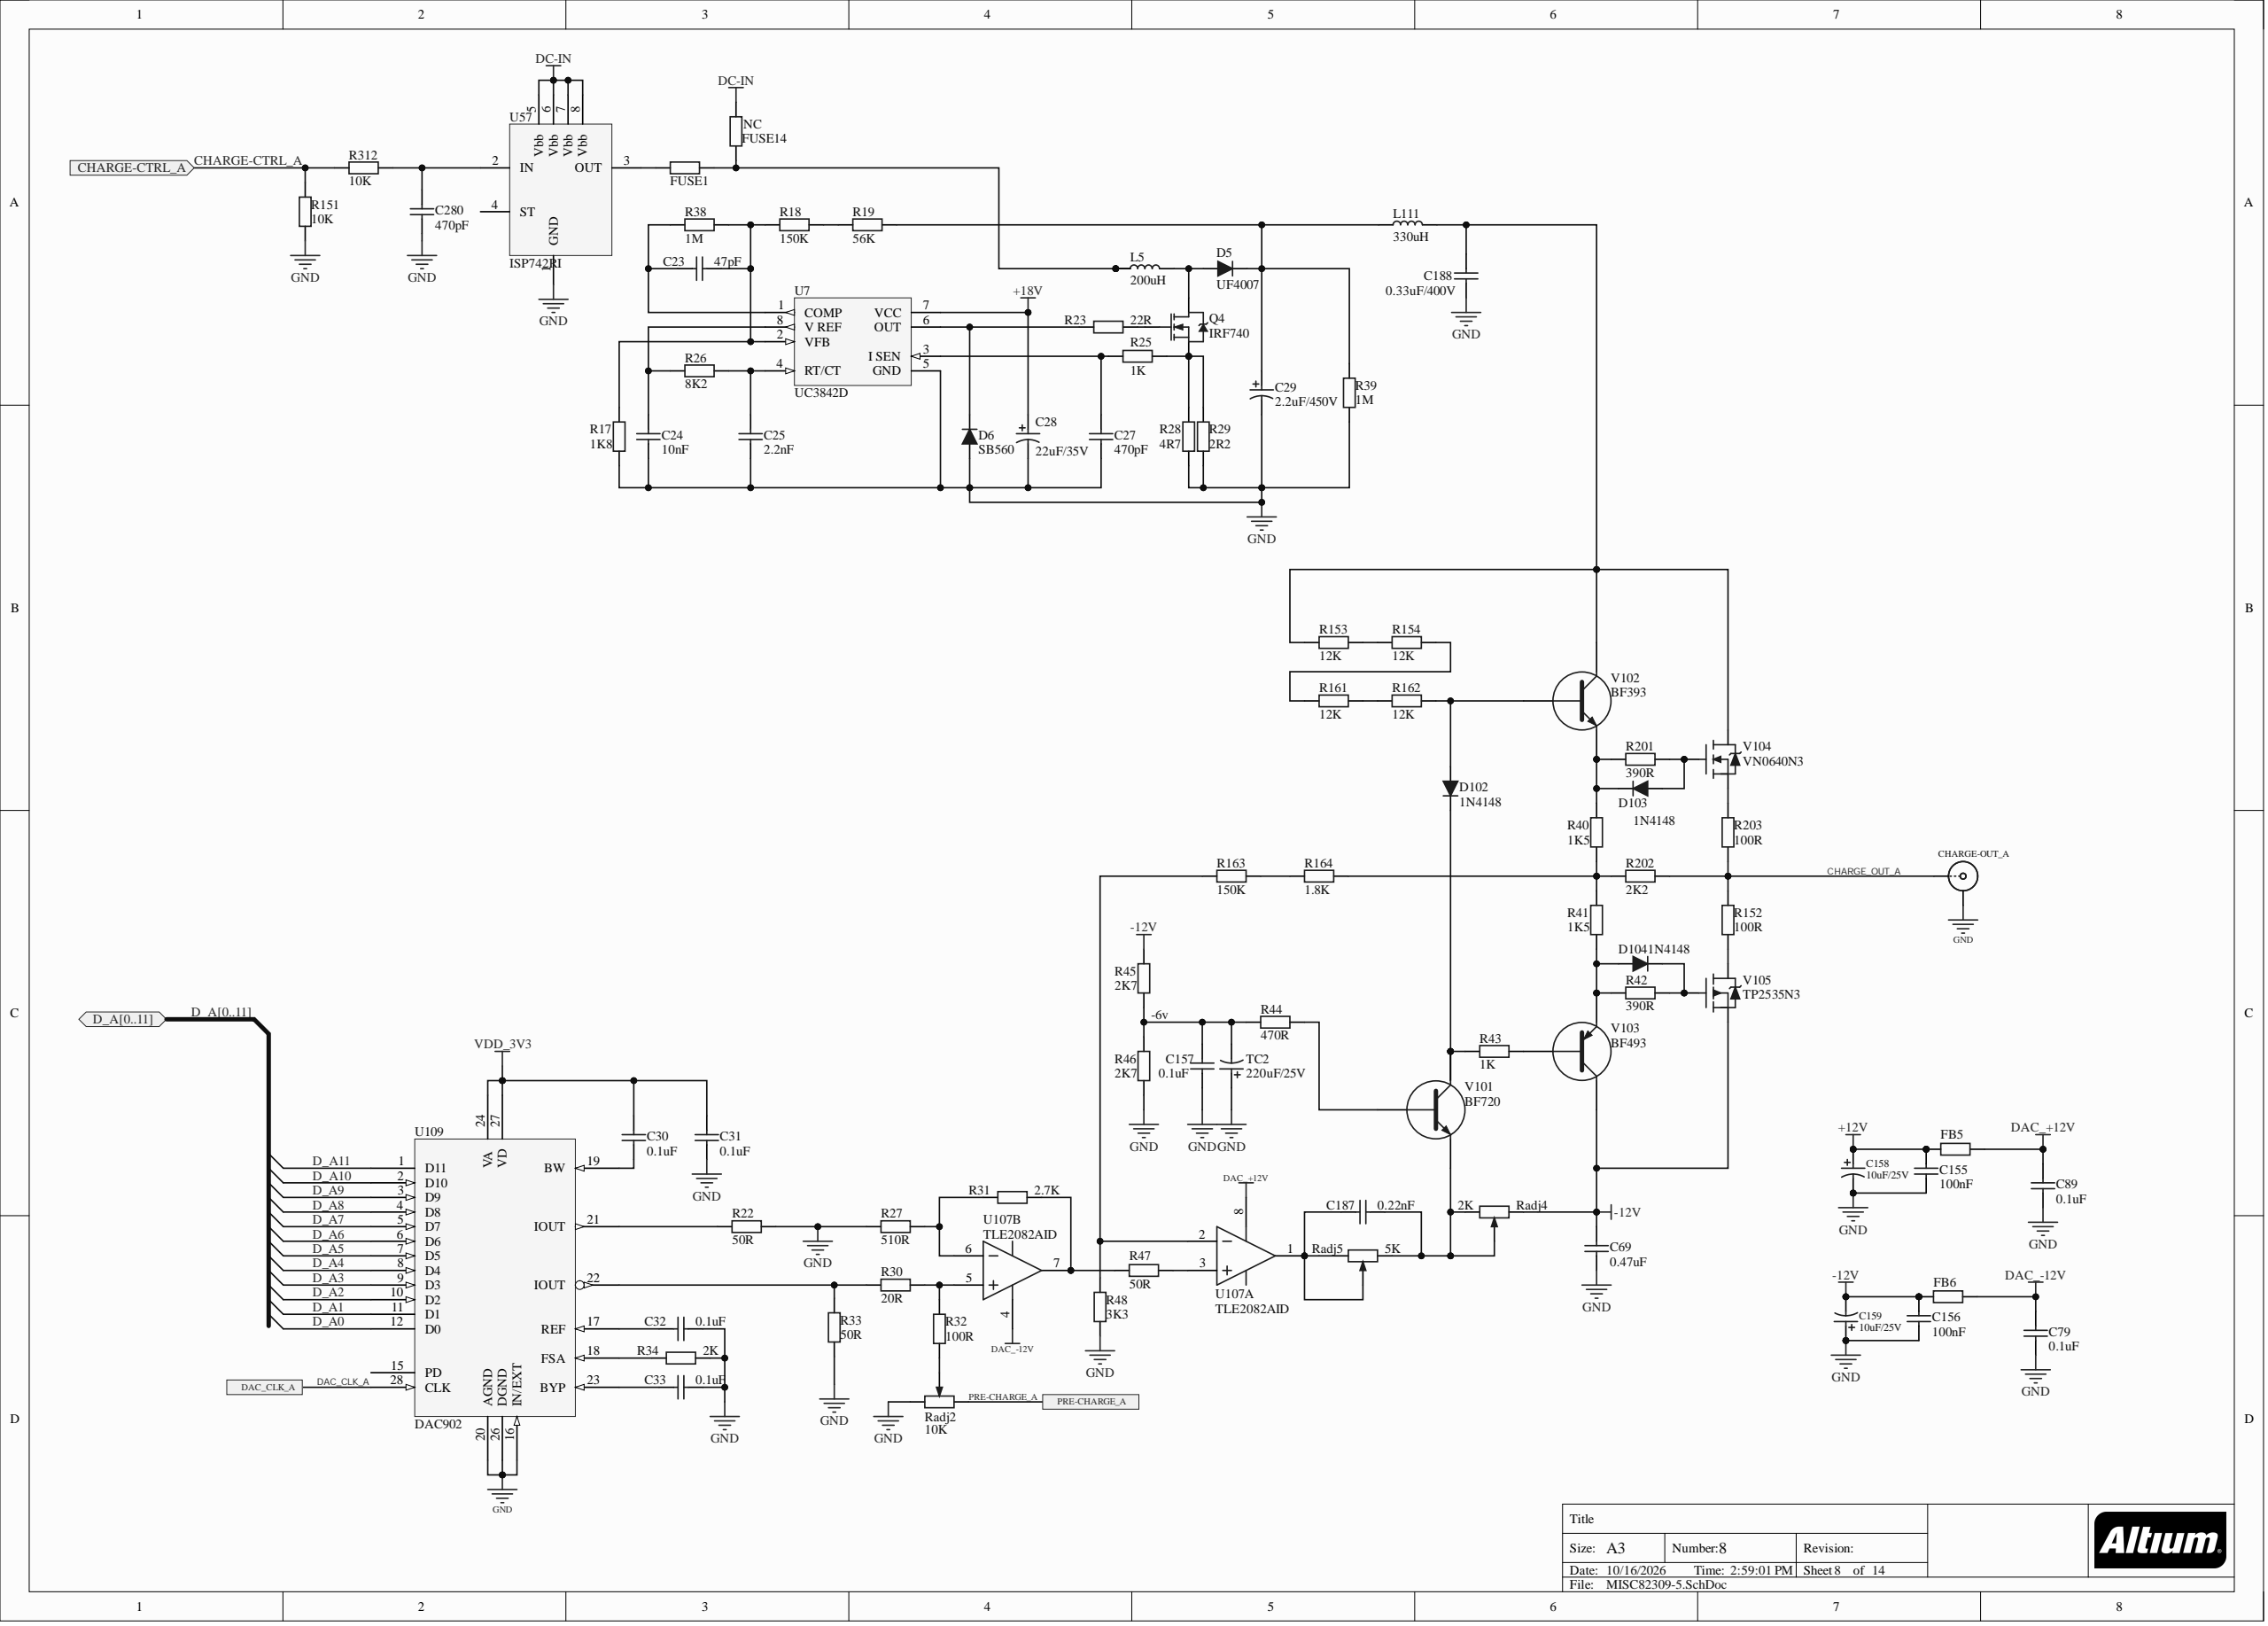Circuit board | Altium Designer | 747 parts | 576 nets | one sheet of the schematic
Parts on this sheet (reference | value | footprint):
C23 | 47pF | C1206
C24 | 10nF | C1206
C25 | 2.2nF | C1206
C27 | 470pF | C1206
C28 | 22uF/35V | E6.3X5.4
C29 | 2.2uF/450V | CAP-EL-10X13_5-5
C30 | 0.1uF | CAP_0805
C31 | 0.1uF | CAP_0805
C32 | 0.1uF | CAP_0805
C33 | 0.1uF | CAP_0805
C69 | 0.47uF | C1206
C79 | 0.1uF | C0805
C89 | 0.1uF | C0805
C155 | 100nF | C0805
C156 | 100nF | C0805
C157 | 0.1uF | CAP_0805
C158 | 10uF/25V | E5X5.4
C159 | 10uF/25V | E5X5.4
C187 | 0.22nF | CAP_0805
C188 | 0.33uF/400V | CBB-400V-10mm
C280 | 470pF | C0603
CHARGE-OUT_A | SMB | SMB_V-RJ45
D102 | 1N4148 | DO-213AA
D103 | 1N4148 | DO-213AA
FB5 | 60 | SMD0805-L
FB6 | 60 | SMD0805-L
FUSE1 | ASMD050-1812(30V,0.5A) | SMD1812-Fuse
FUSE14 | ASMD050-1812(30V,0.5A) | SMD1812-Fuse
L5 | 200uH | L200/1.4A
L111 | 330uH | L-9x12
Q4 | IRF740 | TO220V1
R17 | 1K8 | R1206
R18 | 150K | R1206
R19 | 56K | R1206
R22 | 50R | RES_0805
R23 | 22R | R1206
R25 | 1K | R1206
R26 | 8K2 | R1206
R27 | 510R | RES_0805
R28 | 4R7 | R1206
R29 | 2R2 | R1206
R30 | 20R | RES_0805
R31 | 2.7K | RES_0805
R32 | 100R | RES_0805
R33 | 50R | RES_0805
R34 | 2K | RES_0805
R38 | 1M | R1206
R39 | 1M | R1206
R40 | 1K5 | R1206
R41 | 1K5 | R1206
R42 | 390R | R1206
R43 | 1K | R1206
R44 | 470R | RES_0805
R45 | 2K7 | RES_0805
R46 | 2K7 | RES_0805
R47 | 50R | RES_0805
R48 | 3K3 | RES_0805
R151 | 10K | R0603
R152 | 100R | R1206
R153 | 12K | R1206
R154 | 12K | R1206
R161 | 12K | R1206
R162 | 12K | R1206
R163 | 150K | R1206
R164 | 1.8K | R1206
R201 | 390R | R1206
R202 | 2K2 | R1206
R203 | 100R | R1206
R312 | 10K | R0603
Radj2 | 10K | Radj
Radj4 | 2K | Radj
Radj5 | 5K | Radj
TC2 | 220uF/25V | E8X10,2
U7 | UC3842D | SOIC-8
U57 | ISP742RI | P-DSO-8
U109 | DAC902 | SOP127P1020X265-28N
V101 | BF720 | SOT223
V102 | BF393 | TO-92
V103 | BF493 | TO-92
V104 | VN0640N3 | TO-92
V105 | TP2535N3 | TO-92
Nets of these parts (net: part-pin ...):
VDD_3V3: C30-1 C31-1 U109-24 U109-27
PRE-CHARGE_A: Radj2-1
NetR203_1: R203-1 V104-1
NetR163_1: R163-1 R164-2
NetR161_1: R161-1 R162-2
NetR154_1: R154-1 R161-2
NetR153_1: R153-1 R154-2
NetR152_2: R152-2 V105-1
NetR48_2: R48-2 R163-2
NetR47_2: R47-2
NetR44_1: R44-1 V101-1
NetR43_1: R43-1 V103-2
NetR40_2: R40-2 R41-1 R164-1 R202-1
NetR34_1: R34-1 U109-18
NetR32_1: R32-1 Radj2-2
NetR31_2: R31-2 R47-1
NetR30_2: R30-2 R32-2
NetR30_1: R30-1 R33-2 U109-22
NetR27_2: R27-2 R31-1
NetR22_1: R22-1 U109-21
NetR18_2: R18-2 R19-1
NetQ4_3: Q4-3 R25-2 R28-2 R29-2
NetQ4_1: Q4-1 R23-2
NetFUSE1_2: FUSE1-2 FUSE14-2 L5-1 L5-3
NetFUSE1_1: FUSE1-1 U57-3
NetD104_2: R42-2 V105-2
NetD104_1: R41-2 R42-1 V103-1
NetD103_2: D103-2 R40-1 R201-1 V102-1
NetD103_1: D103-1 R201-2 V104-2
NetD102_2: D102-2 R43-2 V101-2 V101-4
NetD102_1: D102-1 R162-1 V102-2
NetD6_2: R23-1 U7-6
NetD5_1: L5-2 Q4-2
NetC280_2: C280-2 R312-1 U57-2
NetC188_2: C188-2 L111-2 R153-2 V102-3 V104-3
NetC187_2: C187-2 Radj5-1 Radj5-2
NetC187_1: C187-1 Radj4-1 Radj4-2 Radj5-3 V101-3
NetC157_1: C157-1 R44-2 R45-2 R46-1 TC2-2
NetC33_2: C33-2 U109-23
NetC32_1: C32-1 U109-17
NetC30_2: C30-2 U109-19
NetC29_1: C29-1 L111-1 R19-2 R39-2
NetC27_1: C27-1 R25-1 U7-3
NetC25_1: C25-1 R26-2 U7-4
NetC24_1: C24-1 R26-1 U7-8
NetC23_2: C23-2 R38-1 U7-1
NetC23_1: C23-1 R17-2 R18-1 R38-2 U7-2
GND: C24-2 C25-2 C27-2 C28-2 C29-2 C31-2 C32-2 C33-1 C69-2 C79-1 C89-1 C155-2 C156-2 C157-2 C158-2 C159-1 C188-1 C280-1 CHARGE-OUT_A-2 R17-1 R22-2 R27-1 R28-1 R29-1 R33-1 R34-2 R39-1 R46-2 R48-1 R151-1 Radj2-3 TC2-1 U7-5 U57-1 U109-16 U109-20 U109-26
DC-IN: FUSE14-1 U57-5 U57-6 U57-7 U57-8
DAC_CLK_A: U109-28
DAC_-12V: C79-2 FB6-2
DAC_+12V: C89-2 FB5-2
D_A11: U109-1
D_A10: U109-2
D_A9: U109-3
D_A8: U109-4
D_A7: U109-5
D_A6: U109-6
D_A5: U109-7
D_A4: U109-8
D_A3: U109-9
D_A2: U109-10
D_A1: U109-11
D_A0: U109-12
CHARGE_OUT_A: CHARGE-OUT_A-1 R152-1 R202-2 R203-2
CHARGE-CTRL_A: R151-2 R312-2
-12V: C69-1 C156-1 C159-2 FB6-1 R45-1 Radj4-3 V103-3 V105-3
+18V: C28-1 U7-7
+12V: C155-1 C158-1 FB5-1